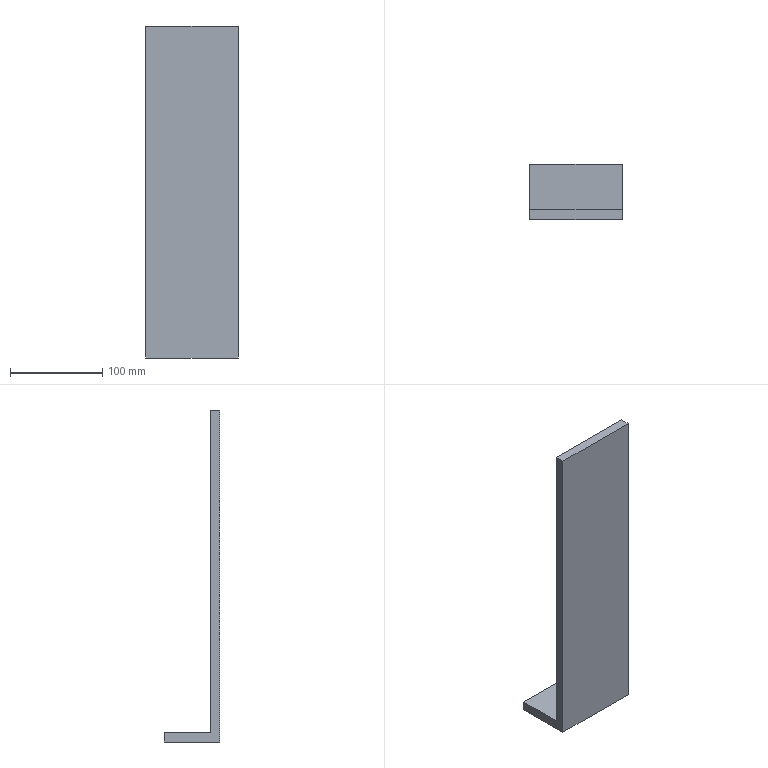Part | STEP file | Part 10 | 1 solid | 8 faces | box 100 x 60 x 360 mm | volume 410000 mm3 | plane 8
STEP:
#1=CARTESIAN_POINT('',(50.,-30.,0.));
#2=VERTEX_POINT('',#1);
#3=CARTESIAN_POINT('',(50.,30.,0.));
#4=VERTEX_POINT('',#3);
#5=CARTESIAN_POINT('',(50.,30.,0.));
#6=DIRECTION('',(0.,1.,0.));
#7=VECTOR('',#6,1000.);
#8=LINE('',#5,#7);
#9=EDGE_CURVE('',#2,#4,#8,.T.);
#10=ORIENTED_EDGE('',*,*,#9,.T.);
#11=CARTESIAN_POINT('',(50.,30.,10.));
#12=VERTEX_POINT('',#11);
#13=CARTESIAN_POINT('',(50.,30.,10.));
#14=DIRECTION('',(0.,0.,-1.));
#15=VECTOR('',#14,1000.);
#16=LINE('',#13,#15);
#17=EDGE_CURVE('',#12,#4,#16,.T.);
#18=ORIENTED_EDGE('',*,*,#17,.F.);
#19=CARTESIAN_POINT('',(50.,-20.,10.));
#20=VERTEX_POINT('',#19);
#21=CARTESIAN_POINT('',(50.,30.,10.));
#22=DIRECTION('',(0.,1.,0.));
#23=VECTOR('',#22,1000.);
#24=LINE('',#21,#23);
#25=EDGE_CURVE('',#20,#12,#24,.T.);
#26=ORIENTED_EDGE('',*,*,#25,.F.);
#27=CARTESIAN_POINT('',(50.,-20.,360.));
#28=VERTEX_POINT('',#27);
#29=CARTESIAN_POINT('',(50.,-20.,360.));
#30=DIRECTION('',(0.,0.,-1.));
#31=VECTOR('',#30,1000.);
#32=LINE('',#29,#31);
#33=EDGE_CURVE('',#28,#20,#32,.T.);
#34=ORIENTED_EDGE('',*,*,#33,.F.);
#35=CARTESIAN_POINT('',(50.,-30.,360.));
#36=VERTEX_POINT('',#35);
#37=CARTESIAN_POINT('',(50.,-30.,360.));
#38=DIRECTION('',(0.,1.,0.));
#39=VECTOR('',#38,1000.);
#40=LINE('',#37,#39);
#41=EDGE_CURVE('',#36,#28,#40,.T.);
#42=ORIENTED_EDGE('',*,*,#41,.F.);
#43=CARTESIAN_POINT('',(50.,-30.,10.));
#44=DIRECTION('',(0.,0.,-1.));
#45=VECTOR('',#44,1000.);
#46=LINE('',#43,#45);
#47=EDGE_CURVE('',#36,#2,#46,.T.);
#48=ORIENTED_EDGE('',*,*,#47,.T.);
#49=EDGE_LOOP('',(#10,#18,#26,#34,#42,#48));
#50=FACE_OUTER_BOUND('',#49,.T.);
#51=CARTESIAN_POINT('',(50.,30.,10.));
#52=DIRECTION('',(-1.,0.,0.));
#53=DIRECTION('',(0.,-1.,0.));
#54=AXIS2_PLACEMENT_3D('',#51,#52,#53);
#55=PLANE('',#54);
#56=ADVANCED_FACE('',(#50),#55,.F.);
#57=CARTESIAN_POINT('',(-50.,30.,0.));
#58=VERTEX_POINT('',#57);
#59=CARTESIAN_POINT('',(-50.,30.,0.));
#60=DIRECTION('',(-1.,0.,0.));
#61=VECTOR('',#60,1000.);
#62=LINE('',#59,#61);
#63=EDGE_CURVE('',#4,#58,#62,.T.);
#64=ORIENTED_EDGE('',*,*,#63,.T.);
#65=CARTESIAN_POINT('',(-50.,30.,10.));
#66=VERTEX_POINT('',#65);
#67=CARTESIAN_POINT('',(-50.,30.,10.));
#68=DIRECTION('',(0.,0.,-1.));
#69=VECTOR('',#68,1000.);
#70=LINE('',#67,#69);
#71=EDGE_CURVE('',#66,#58,#70,.T.);
#72=ORIENTED_EDGE('',*,*,#71,.F.);
#73=CARTESIAN_POINT('',(-50.,30.,10.));
#74=DIRECTION('',(-1.,0.,0.));
#75=VECTOR('',#74,1000.);
#76=LINE('',#73,#75);
#77=EDGE_CURVE('',#12,#66,#76,.T.);
#78=ORIENTED_EDGE('',*,*,#77,.F.);
#79=ORIENTED_EDGE('',*,*,#17,.T.);
#80=EDGE_LOOP('',(#64,#72,#78,#79));
#81=FACE_OUTER_BOUND('',#80,.T.);
#82=CARTESIAN_POINT('',(-50.,30.,10.));
#83=DIRECTION('',(0.,-1.,0.));
#84=DIRECTION('',(0.,0.,-1.));
#85=AXIS2_PLACEMENT_3D('',#82,#83,#84);
#86=PLANE('',#85);
#87=ADVANCED_FACE('',(#81),#86,.F.);
#88=CARTESIAN_POINT('',(-50.,-30.,0.));
#89=VERTEX_POINT('',#88);
#90=CARTESIAN_POINT('',(-50.,30.,0.));
#91=DIRECTION('',(0.,-1.,0.));
#92=VECTOR('',#91,1000.);
#93=LINE('',#90,#92);
#94=EDGE_CURVE('',#58,#89,#93,.T.);
#95=ORIENTED_EDGE('',*,*,#94,.T.);
#96=CARTESIAN_POINT('',(-50.,-30.,360.));
#97=VERTEX_POINT('',#96);
#98=CARTESIAN_POINT('',(-50.,-30.,10.));
#99=DIRECTION('',(0.,0.,-1.));
#100=VECTOR('',#99,1000.);
#101=LINE('',#98,#100);
#102=EDGE_CURVE('',#97,#89,#101,.T.);
#103=ORIENTED_EDGE('',*,*,#102,.F.);
#104=CARTESIAN_POINT('',(-50.,-20.,360.));
#105=VERTEX_POINT('',#104);
#106=CARTESIAN_POINT('',(-50.,-30.,360.));
#107=DIRECTION('',(0.,-1.,0.));
#108=VECTOR('',#107,1000.);
#109=LINE('',#106,#108);
#110=EDGE_CURVE('',#105,#97,#109,.T.);
#111=ORIENTED_EDGE('',*,*,#110,.F.);
#112=CARTESIAN_POINT('',(-50.,-20.,10.));
#113=VERTEX_POINT('',#112);
#114=CARTESIAN_POINT('',(-50.,-20.,360.));
#115=DIRECTION('',(0.,0.,-1.));
#116=VECTOR('',#115,1000.);
#117=LINE('',#114,#116);
#118=EDGE_CURVE('',#105,#113,#117,.T.);
#119=ORIENTED_EDGE('',*,*,#118,.T.);
#120=CARTESIAN_POINT('',(-50.,30.,10.));
#121=DIRECTION('',(0.,-1.,0.));
#122=VECTOR('',#121,1000.);
#123=LINE('',#120,#122);
#124=EDGE_CURVE('',#66,#113,#123,.T.);
#125=ORIENTED_EDGE('',*,*,#124,.F.);
#126=ORIENTED_EDGE('',*,*,#71,.T.);
#127=EDGE_LOOP('',(#95,#103,#111,#119,#125,#126));
#128=FACE_OUTER_BOUND('',#127,.T.);
#129=CARTESIAN_POINT('',(-50.,30.,10.));
#130=DIRECTION('',(1.,0.,0.));
#131=DIRECTION('',(0.,1.,0.));
#132=AXIS2_PLACEMENT_3D('',#129,#130,#131);
#133=PLANE('',#132);
#134=ADVANCED_FACE('',(#128),#133,.F.);
#135=CARTESIAN_POINT('',(-50.,-30.,0.));
#136=DIRECTION('',(1.,0.,0.));
#137=VECTOR('',#136,1000.);
#138=LINE('',#135,#137);
#139=EDGE_CURVE('',#89,#2,#138,.T.);
#140=ORIENTED_EDGE('',*,*,#139,.T.);
#141=ORIENTED_EDGE('',*,*,#47,.F.);
#142=CARTESIAN_POINT('',(-50.,-30.,360.));
#143=DIRECTION('',(1.,0.,0.));
#144=VECTOR('',#143,1000.);
#145=LINE('',#142,#144);
#146=EDGE_CURVE('',#97,#36,#145,.T.);
#147=ORIENTED_EDGE('',*,*,#146,.F.);
#148=ORIENTED_EDGE('',*,*,#102,.T.);
#149=EDGE_LOOP('',(#140,#141,#147,#148));
#150=FACE_OUTER_BOUND('',#149,.T.);
#151=CARTESIAN_POINT('',(-50.,-30.,10.));
#152=DIRECTION('',(0.,1.,0.));
#153=DIRECTION('',(0.,0.,1.));
#154=AXIS2_PLACEMENT_3D('',#151,#152,#153);
#155=PLANE('',#154);
#156=ADVANCED_FACE('',(#150),#155,.F.);
#157=CARTESIAN_POINT('',(-50.,-20.,10.));
#158=DIRECTION('',(-1.,0.,0.));
#159=VECTOR('',#158,1000.);
#160=LINE('',#157,#159);
#161=EDGE_CURVE('',#20,#113,#160,.T.);
#162=ORIENTED_EDGE('',*,*,#161,.F.);
#163=ORIENTED_EDGE('',*,*,#25,.T.);
#164=ORIENTED_EDGE('',*,*,#77,.T.);
#165=ORIENTED_EDGE('',*,*,#124,.T.);
#166=EDGE_LOOP('',(#162,#163,#164,#165));
#167=FACE_OUTER_BOUND('',#166,.T.);
#168=CARTESIAN_POINT('',(0.,0.,10.));
#169=DIRECTION('',(0.,0.,1.));
#170=DIRECTION('',(1.,0.,0.));
#171=AXIS2_PLACEMENT_3D('',#168,#169,#170);
#172=PLANE('',#171);
#173=ADVANCED_FACE('',(#167),#172,.T.);
#174=ORIENTED_EDGE('',*,*,#9,.F.);
#175=ORIENTED_EDGE('',*,*,#139,.F.);
#176=ORIENTED_EDGE('',*,*,#94,.F.);
#177=ORIENTED_EDGE('',*,*,#63,.F.);
#178=EDGE_LOOP('',(#174,#175,#176,#177));
#179=FACE_OUTER_BOUND('',#178,.T.);
#180=CARTESIAN_POINT('',(0.,0.,0.));
#181=DIRECTION('',(0.,0.,1.));
#182=DIRECTION('',(1.,0.,0.));
#183=AXIS2_PLACEMENT_3D('',#180,#181,#182);
#184=PLANE('',#183);
#185=ADVANCED_FACE('',(#179),#184,.F.);
#186=ORIENTED_EDGE('',*,*,#161,.T.);
#187=ORIENTED_EDGE('',*,*,#118,.F.);
#188=CARTESIAN_POINT('',(-50.,-20.,360.));
#189=DIRECTION('',(-1.,0.,0.));
#190=VECTOR('',#189,1000.);
#191=LINE('',#188,#190);
#192=EDGE_CURVE('',#28,#105,#191,.T.);
#193=ORIENTED_EDGE('',*,*,#192,.F.);
#194=ORIENTED_EDGE('',*,*,#33,.T.);
#195=EDGE_LOOP('',(#186,#187,#193,#194));
#196=FACE_OUTER_BOUND('',#195,.T.);
#197=CARTESIAN_POINT('',(-50.,-20.,360.));
#198=DIRECTION('',(0.,-1.,0.));
#199=DIRECTION('',(0.,0.,-1.));
#200=AXIS2_PLACEMENT_3D('',#197,#198,#199);
#201=PLANE('',#200);
#202=ADVANCED_FACE('',(#196),#201,.F.);
#203=ORIENTED_EDGE('',*,*,#110,.T.);
#204=ORIENTED_EDGE('',*,*,#146,.T.);
#205=ORIENTED_EDGE('',*,*,#41,.T.);
#206=ORIENTED_EDGE('',*,*,#192,.T.);
#207=EDGE_LOOP('',(#203,#204,#205,#206));
#208=FACE_OUTER_BOUND('',#207,.T.);
#209=CARTESIAN_POINT('',(0.,0.,360.));
#210=DIRECTION('',(0.,0.,-1.));
#211=DIRECTION('',(-1.,0.,0.));
#212=AXIS2_PLACEMENT_3D('',#209,#210,#211);
#213=PLANE('',#212);
#214=ADVANCED_FACE('',(#208),#213,.F.);
#215=CLOSED_SHELL('',(#56,#87,#134,#156,#173,#185,#202,#214));
#216=MANIFOLD_SOLID_BREP('',#215);
#217=CARTESIAN_POINT('',(0.,0.,0.));
#218=DIRECTION('',(0.,0.,1.));
#219=DIRECTION('',(1.,0.,0.));
#220=AXIS2_PLACEMENT_3D('',#217,#218,#219);
#221=(LENGTH_UNIT()NAMED_UNIT(*)SI_UNIT(.MILLI.,.METRE.));
#222=UNCERTAINTY_MEASURE_WITH_UNIT(LENGTH_MEASURE(0.00001),#221,'','');
#223=(NAMED_UNIT(*)PLANE_ANGLE_UNIT()SI_UNIT($,.RADIAN.));
#224=(NAMED_UNIT(*)SI_UNIT($,.STERADIAN.)SOLID_ANGLE_UNIT());
#225=(GEOMETRIC_REPRESENTATION_CONTEXT(3)GLOBAL_UNCERTAINTY_ASSIGNED_CONTEXT((#222))GLOBAL_UNIT_ASSIGNED_CONTEXT((#221,#223,#224))REPRESENTATION_CONTEXT('',''));
#226=ADVANCED_BREP_SHAPE_REPRESENTATION('',(#216,#220),#225);